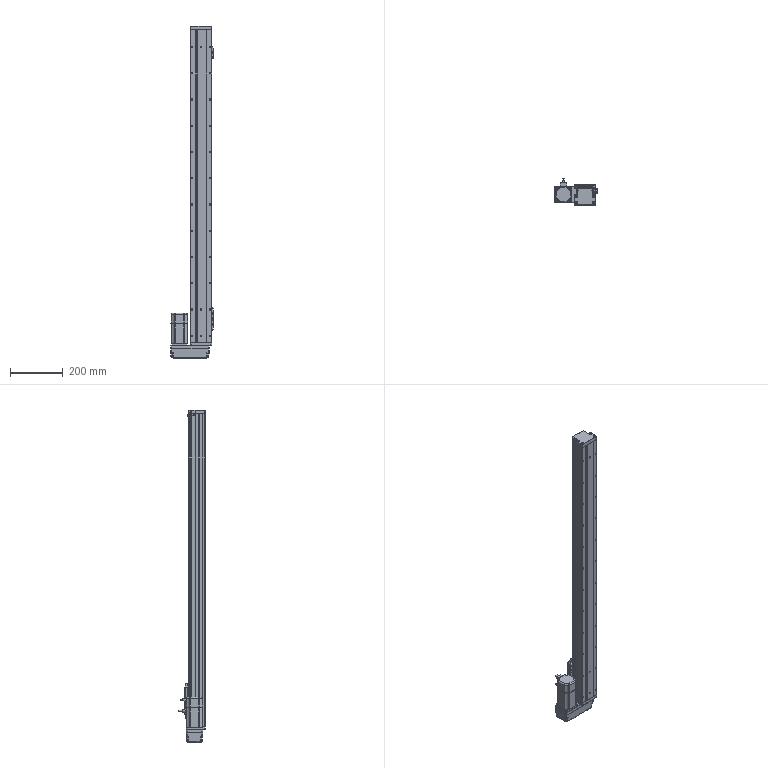Part | NX | features BREP 20 | 49 solids | 2084 faces | box 162 x 101.5 x 1265 mm | volume 3954942 mm3 | plane 831 | cylinder 700 | cone 351 | torus 92 | spline 73 | sphere 37 | commonest cylinder face diameters 4 x75 5 x75 1 x51 2.5 x48 5.4 x48 0.4 x42